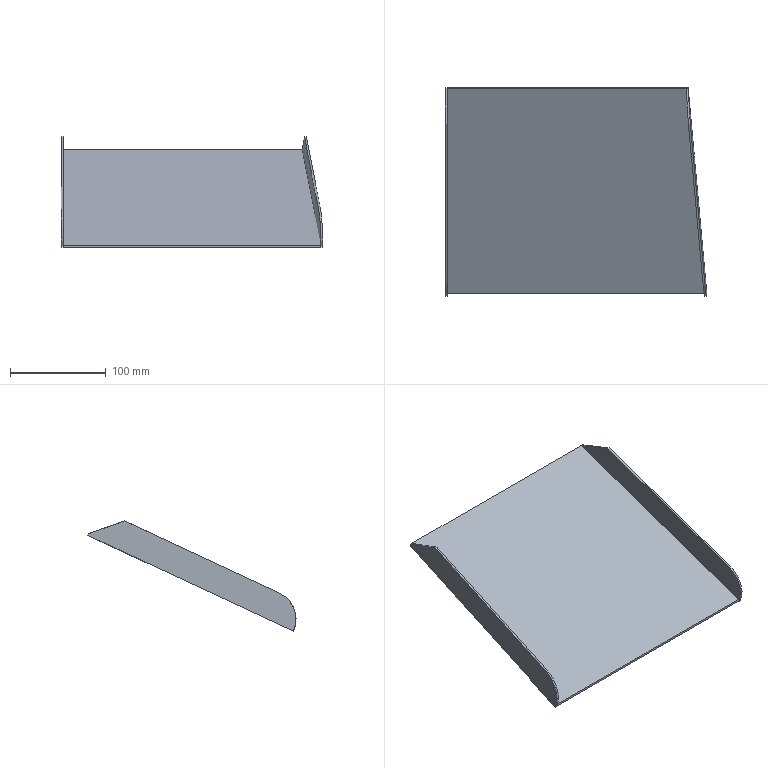Part | NX | features solid 2 | 1 solid | 15 faces | box 273.716 x 217.701 x 115.597 mm | volume 149004 mm3 | plane 12 | cylinder 2 | spline 1 | commonest cylinder face diameters 60 x2
STEP:
#1=CARTESIAN_POINT('',(382.,-625.361,-199.495));
#2=VERTEX_POINT('',#1);
#3=CARTESIAN_POINT('',(634.106,-625.268,-199.451));
#4=VERTEX_POINT('',#3);
#5=CARTESIAN_POINT('',(634.106,-625.268,-199.451));
#6=CARTESIAN_POINT('',(548.539,-625.34,-199.485));
#7=CARTESIAN_POINT('',(464.504,-625.371,-199.499));
#8=CARTESIAN_POINT('',(382.,-625.361,-199.495));
#9=B_SPLINE_CURVE_WITH_KNOTS('',3,(#5,#6,#7,#8),.UNSPECIFIED.,.F.,.F.,(4,4),(0.,0.992),.UNSPECIFIED.);
#10=EDGE_CURVE('',#2,#4,#9,.F.);
#11=ORIENTED_EDGE('',*,*,#10,.F.);
#12=CARTESIAN_POINT('',(382.,-626.207,-197.682));
#13=VERTEX_POINT('',#12);
#14=CARTESIAN_POINT('',(382.,-626.206,-197.682));
#15=CARTESIAN_POINT('',(382.,-625.925,-198.286));
#16=CARTESIAN_POINT('',(382.,-625.643,-198.89));
#17=CARTESIAN_POINT('',(382.,-625.361,-199.495));
#18=B_SPLINE_CURVE_WITH_KNOTS('',3,(#14,#15,#16,#17),.UNSPECIFIED.,.F.,.F.,(4,4),(0.,1.),.UNSPECIFIED.);
#19=EDGE_CURVE('',#2,#13,#18,.F.);
#20=ORIENTED_EDGE('',*,*,#19,.T.);
#21=CARTESIAN_POINT('',(634.106,-626.113,-197.638));
#22=VERTEX_POINT('',#21);
#23=CARTESIAN_POINT('',(634.106,-626.113,-197.638));
#24=CARTESIAN_POINT('',(548.539,-626.185,-197.672));
#25=CARTESIAN_POINT('',(464.504,-626.217,-197.687));
#26=CARTESIAN_POINT('',(382.,-626.207,-197.682));
#27=B_SPLINE_CURVE_WITH_KNOTS('',3,(#23,#24,#25,#26),.UNSPECIFIED.,.F.,.F.,(4,4),(0.,0.992),.UNSPECIFIED.);
#28=EDGE_CURVE('',#13,#22,#27,.F.);
#29=ORIENTED_EDGE('',*,*,#28,.T.);
#30=CARTESIAN_POINT('',(634.106,-625.268,-199.451));
#31=CARTESIAN_POINT('',(634.106,-625.55,-198.847));
#32=CARTESIAN_POINT('',(634.106,-625.831,-198.243));
#33=CARTESIAN_POINT('',(634.106,-626.113,-197.638));
#34=B_SPLINE_CURVE_WITH_KNOTS('',3,(#30,#31,#32,#33),.UNSPECIFIED.,.F.,.F.,(4,4),(0.,1.),.UNSPECIFIED.);
#35=EDGE_CURVE('',#22,#4,#34,.F.);
#36=ORIENTED_EDGE('',*,*,#35,.T.);
#37=EDGE_LOOP('',(#11,#20,#29,#36));
#38=FACE_BOUND('',#37,.T.);
#39=CARTESIAN_POINT('',(634.106,-626.113,-197.638));
#40=CARTESIAN_POINT('',(634.106,-625.268,-199.451));
#41=CARTESIAN_POINT('',(548.539,-626.185,-197.672));
#42=CARTESIAN_POINT('',(548.539,-625.34,-199.485));
#43=CARTESIAN_POINT('',(464.504,-626.217,-197.687));
#44=CARTESIAN_POINT('',(464.504,-625.371,-199.499));
#45=CARTESIAN_POINT('',(382.,-626.207,-197.682));
#46=CARTESIAN_POINT('',(382.,-625.361,-199.495));
#47=B_SPLINE_SURFACE_WITH_KNOTS('',3,1,((#39,#40),(#41,#42),(#43,#44),(#45,#46)),.SURF_OF_LINEAR_EXTRUSION.,.F.,.F.,.F.,(4,4),(2,2),(0.,0.992),(0.,1.),.PIECEWISE_BEZIER_KNOTS.);
#48=ADVANCED_FACE('',(#38),#47,.F.);
#49=CARTESIAN_POINT('',(382.,-840.,-299.582));
#50=VERTEX_POINT('',#49);
#51=CARTESIAN_POINT('',(382.,-840.,-297.376));
#52=VERTEX_POINT('',#51);
#53=CARTESIAN_POINT('',(382.,-840.,-720.));
#54=DIRECTION('',(0.,0.,1.));
#55=VECTOR('',#54,1000.);
#56=LINE('',#53,#55);
#57=EDGE_CURVE('',#50,#52,#56,.T.);
#58=ORIENTED_EDGE('',*,*,#57,.F.);
#59=CARTESIAN_POINT('',(651.709,-840.,-299.582));
#60=VERTEX_POINT('',#59);
#61=CARTESIAN_POINT('',(-476.248,-840.,-299.582));
#62=DIRECTION('',(1.,0.,0.));
#63=VECTOR('',#62,1000.);
#64=LINE('',#61,#63);
#65=EDGE_CURVE('',#50,#60,#64,.T.);
#66=ORIENTED_EDGE('',*,*,#65,.T.);
#67=CARTESIAN_POINT('',(651.632,-840.,-297.376));
#68=VERTEX_POINT('',#67);
#69=CARTESIAN_POINT('',(665.018,-840.,-680.08));
#70=DIRECTION('',(-0.03496,0.,0.9994));
#71=VECTOR('',#70,1000.);
#72=LINE('',#69,#71);
#73=EDGE_CURVE('',#60,#68,#72,.T.);
#74=ORIENTED_EDGE('',*,*,#73,.T.);
#75=CARTESIAN_POINT('',(-476.248,-840.,-297.376));
#76=DIRECTION('',(1.,0.,0.));
#77=VECTOR('',#76,1000.);
#78=LINE('',#75,#77);
#79=EDGE_CURVE('',#52,#68,#78,.T.);
#80=ORIENTED_EDGE('',*,*,#79,.F.);
#81=EDGE_LOOP('',(#58,#66,#74,#80));
#82=FACE_BOUND('',#81,.T.);
#83=CARTESIAN_POINT('',(-476.248,-840.,-720.));
#84=DIRECTION('',(0.,1.,0.));
#85=DIRECTION('',(-1.,0.,0.));
#86=AXIS2_PLACEMENT_3D('',#83,#84,#85);
#87=PLANE('',#86);
#88=ADVANCED_FACE('',(#82),#87,.F.);
#89=ORIENTED_EDGE('',*,*,#28,.F.);
#90=CARTESIAN_POINT('',(382.,-651.161,-209.318));
#91=DIRECTION('',(0.,-0.9063,-0.4226));
#92=VECTOR('',#91,1000.);
#93=LINE('',#90,#92);
#94=EDGE_CURVE('',#13,#52,#93,.T.);
#95=ORIENTED_EDGE('',*,*,#94,.T.);
#96=ORIENTED_EDGE('',*,*,#79,.T.);
#97=CARTESIAN_POINT('',(632.113,-626.263,-197.708));
#98=VERTEX_POINT('',#97);
#99=CARTESIAN_POINT('',(621.843,-513.811,-145.271));
#100=DIRECTION('',(0.08249,-0.9032,-0.4212));
#101=VECTOR('',#100,1000.);
#102=LINE('',#99,#101);
#103=EDGE_CURVE('',#98,#68,#102,.T.);
#104=ORIENTED_EDGE('',*,*,#103,.F.);
#105=CARTESIAN_POINT('',(634.106,-626.113,-197.638));
#106=DIRECTION('',(0.9966,0.07476,0.03486));
#107=VECTOR('',#106,1000.);
#108=LINE('',#105,#107);
#109=EDGE_CURVE('',#98,#22,#108,.T.);
#110=ORIENTED_EDGE('',*,*,#109,.T.);
#111=EDGE_LOOP('',(#89,#95,#96,#104,#110));
#112=FACE_BOUND('',#111,.T.);
#113=CARTESIAN_POINT('',(-1209.175,-651.161,-209.318));
#114=DIRECTION('',(0.,-0.4226,0.9063));
#115=DIRECTION('',(1.,0.,0.));
#116=AXIS2_PLACEMENT_3D('',#113,#114,#115);
#117=PLANE('',#116);
#118=ADVANCED_FACE('',(#112),#117,.T.);
#119=CARTESIAN_POINT('',(651.241,-825.582,-259.758));
#120=VERTEX_POINT('',#119);
#121=CARTESIAN_POINT('',(653.716,-840.,-299.582));
#122=VERTEX_POINT('',#121);
#123=CARTESIAN_POINT('',(651.241,-812.903,-286.947));
#124=DIRECTION('',(-0.9966,-0.07476,-0.03486));
#125=DIRECTION('',(0.0748,-0.9972,0.));
#126=AXIS2_PLACEMENT_3D('',#123,#124,#125);
#127=CIRCLE('',#126,30.);
#128=EDGE_CURVE('',#120,#122,#127,.F.);
#129=ORIENTED_EDGE('',*,*,#128,.T.);
#130=CARTESIAN_POINT('',(623.836,-512.816,-147.014));
#131=DIRECTION('',(0.08249,-0.9032,-0.4212));
#132=VECTOR('',#131,1000.);
#133=LINE('',#130,#132);
#134=EDGE_CURVE('',#4,#122,#133,.T.);
#135=ORIENTED_EDGE('',*,*,#134,.F.);
#136=ORIENTED_EDGE('',*,*,#35,.F.);
#137=CARTESIAN_POINT('',(636.415,-663.237,-184.055));
#138=VERTEX_POINT('',#137);
#139=CARTESIAN_POINT('',(636.415,-663.237,-184.055));
#140=DIRECTION('',(-0.05833,0.9375,-0.343));
#141=VECTOR('',#140,1000.);
#142=LINE('',#139,#141);
#143=EDGE_CURVE('',#22,#138,#142,.F.);
#144=ORIENTED_EDGE('',*,*,#143,.T.);
#145=CARTESIAN_POINT('',(634.106,-637.946,-172.262));
#146=DIRECTION('',(0.08249,-0.9032,-0.4212));
#147=VECTOR('',#146,1000.);
#148=LINE('',#145,#147);
#149=EDGE_CURVE('',#138,#120,#148,.T.);
#150=ORIENTED_EDGE('',*,*,#149,.T.);
#151=EDGE_LOOP('',(#129,#135,#136,#144,#150));
#152=FACE_BOUND('',#151,.T.);
#153=CARTESIAN_POINT('',(623.836,-513.661,-145.201));
#154=DIRECTION('',(0.9966,0.07476,0.03486));
#155=DIRECTION('',(-0.0748,0.9972,0.));
#156=AXIS2_PLACEMENT_3D('',#153,#154,#155);
#157=PLANE('',#156);
#158=ADVANCED_FACE('',(#152),#157,.T.);
#159=CARTESIAN_POINT('',(380.,-625.361,-199.495));
#160=VERTEX_POINT('',#159);
#161=CARTESIAN_POINT('',(380.,-840.,-299.582));
#162=VERTEX_POINT('',#161);
#163=CARTESIAN_POINT('',(380.,-650.315,-211.131));
#164=DIRECTION('',(0.,-0.9063,-0.4226));
#165=VECTOR('',#164,1000.);
#166=LINE('',#163,#165);
#167=EDGE_CURVE('',#160,#162,#166,.T.);
#168=ORIENTED_EDGE('',*,*,#167,.T.);
#169=CARTESIAN_POINT('',(380.,-825.489,-259.715));
#170=VERTEX_POINT('',#169);
#171=CARTESIAN_POINT('',(380.,-812.811,-286.904));
#172=DIRECTION('',(-1.,0.,0.));
#173=DIRECTION('',(0.,-1.,0.));
#174=AXIS2_PLACEMENT_3D('',#171,#172,#173);
#175=CIRCLE('',#174,30.);
#176=EDGE_CURVE('',#162,#170,#175,.T.);
#177=ORIENTED_EDGE('',*,*,#176,.T.);
#178=CARTESIAN_POINT('',(380.,-663.416,-184.139));
#179=VERTEX_POINT('',#178);
#180=CARTESIAN_POINT('',(380.,-638.04,-172.305));
#181=DIRECTION('',(0.,-0.9063,-0.4226));
#182=VECTOR('',#181,1000.);
#183=LINE('',#180,#182);
#184=EDGE_CURVE('',#179,#170,#183,.T.);
#185=ORIENTED_EDGE('',*,*,#184,.F.);
#186=CARTESIAN_POINT('',(380.,-626.206,-197.682));
#187=VERTEX_POINT('',#186);
#188=CARTESIAN_POINT('',(380.,-624.877,-198.166));
#189=DIRECTION('',(0.,-0.9397,0.342));
#190=VECTOR('',#189,1000.);
#191=LINE('',#188,#190);
#192=EDGE_CURVE('',#179,#187,#191,.F.);
#193=ORIENTED_EDGE('',*,*,#192,.T.);
#194=CARTESIAN_POINT('',(380.,-626.206,-197.682));
#195=CARTESIAN_POINT('',(380.,-625.925,-198.286));
#196=CARTESIAN_POINT('',(380.,-625.643,-198.89));
#197=CARTESIAN_POINT('',(380.,-625.361,-199.495));
#198=B_SPLINE_CURVE_WITH_KNOTS('',3,(#194,#195,#196,#197),.UNSPECIFIED.,.F.,.F.,(4,4),(0.,1.),.UNSPECIFIED.);
#199=EDGE_CURVE('',#160,#187,#198,.F.);
#200=ORIENTED_EDGE('',*,*,#199,.F.);
#201=EDGE_LOOP('',(#168,#177,#185,#193,#200));
#202=FACE_BOUND('',#201,.T.);
#203=CARTESIAN_POINT('',(380.,-651.161,-209.318));
#204=DIRECTION('',(1.,0.,0.));
#205=DIRECTION('',(0.,1.,0.));
#206=AXIS2_PLACEMENT_3D('',#203,#204,#205);
#207=PLANE('',#206);
#208=ADVANCED_FACE('',(#202),#207,.F.);
#209=CARTESIAN_POINT('',(382.,-625.361,-199.495));
#210=CARTESIAN_POINT('',(381.333,-625.361,-199.495));
#211=CARTESIAN_POINT('',(380.667,-625.361,-199.495));
#212=CARTESIAN_POINT('',(380.,-625.361,-199.495));
#213=B_SPLINE_CURVE_WITH_KNOTS('',3,(#209,#210,#211,#212),.UNSPECIFIED.,.F.,.F.,(4,4),(0.992,1.),.UNSPECIFIED.);
#214=EDGE_CURVE('',#160,#2,#213,.F.);
#215=ORIENTED_EDGE('',*,*,#214,.T.);
#216=ORIENTED_EDGE('',*,*,#10,.T.);
#217=ORIENTED_EDGE('',*,*,#134,.T.);
#218=CARTESIAN_POINT('',(651.723,-840.15,-299.652));
#219=VERTEX_POINT('',#218);
#220=CARTESIAN_POINT('',(653.716,-840.,-299.582));
#221=DIRECTION('',(0.9966,0.07476,0.03486));
#222=VECTOR('',#221,1000.);
#223=LINE('',#220,#222);
#224=EDGE_CURVE('',#122,#219,#223,.F.);
#225=ORIENTED_EDGE('',*,*,#224,.T.);
#226=CARTESIAN_POINT('',(632.113,-625.417,-199.521));
#227=DIRECTION('',(0.08249,-0.9032,-0.4212));
#228=VECTOR('',#227,1000.);
#229=LINE('',#226,#228);
#230=EDGE_CURVE('',#60,#219,#229,.T.);
#231=ORIENTED_EDGE('',*,*,#230,.F.);
#232=ORIENTED_EDGE('',*,*,#65,.F.);
#233=CARTESIAN_POINT('',(-476.248,-840.,-299.582));
#234=DIRECTION('',(1.,0.,0.));
#235=VECTOR('',#234,1000.);
#236=LINE('',#233,#235);
#237=EDGE_CURVE('',#162,#50,#236,.T.);
#238=ORIENTED_EDGE('',*,*,#237,.F.);
#239=ORIENTED_EDGE('',*,*,#167,.F.);
#240=EDGE_LOOP('',(#215,#216,#217,#225,#231,#232,#238,#239));
#241=FACE_BOUND('',#240,.T.);
#242=CARTESIAN_POINT('',(-1209.175,-650.315,-211.131));
#243=DIRECTION('',(0.,-0.4226,0.9063));
#244=DIRECTION('',(1.,0.,0.));
#245=AXIS2_PLACEMENT_3D('',#242,#243,#244);
#246=PLANE('',#245);
#247=ADVANCED_FACE('',(#241),#246,.F.);
#248=ORIENTED_EDGE('',*,*,#73,.F.);
#249=ORIENTED_EDGE('',*,*,#230,.T.);
#250=CARTESIAN_POINT('',(649.248,-825.731,-259.827));
#251=VERTEX_POINT('',#250);
#252=CARTESIAN_POINT('',(649.248,-813.053,-287.017));
#253=DIRECTION('',(-0.9966,-0.07476,-0.03486));
#254=DIRECTION('',(0.0748,-0.9972,0.));
#255=AXIS2_PLACEMENT_3D('',#252,#253,#254);
#256=CIRCLE('',#255,30.);
#257=EDGE_CURVE('',#219,#251,#256,.T.);
#258=ORIENTED_EDGE('',*,*,#257,.T.);
#259=CARTESIAN_POINT('',(634.422,-663.386,-184.125));
#260=VERTEX_POINT('',#259);
#261=CARTESIAN_POINT('',(632.113,-638.096,-172.332));
#262=DIRECTION('',(0.08249,-0.9032,-0.4212));
#263=VECTOR('',#262,1000.);
#264=LINE('',#261,#263);
#265=EDGE_CURVE('',#260,#251,#264,.T.);
#266=ORIENTED_EDGE('',*,*,#265,.F.);
#267=CARTESIAN_POINT('',(632.03,-624.937,-198.193));
#268=DIRECTION('',(0.05833,-0.9375,0.343));
#269=VECTOR('',#268,1000.);
#270=LINE('',#267,#269);
#271=EDGE_CURVE('',#260,#98,#270,.F.);
#272=ORIENTED_EDGE('',*,*,#271,.T.);
#273=ORIENTED_EDGE('',*,*,#103,.T.);
#274=EDGE_LOOP('',(#248,#249,#258,#266,#272,#273));
#275=FACE_BOUND('',#274,.T.);
#276=CARTESIAN_POINT('',(632.113,-625.417,-199.521));
#277=DIRECTION('',(-0.9966,-0.07476,-0.03486));
#278=DIRECTION('',(0.0748,-0.9972,0.));
#279=AXIS2_PLACEMENT_3D('',#276,#277,#278);
#280=PLANE('',#279);
#281=ADVANCED_FACE('',(#275),#280,.T.);
#282=ORIENTED_EDGE('',*,*,#265,.T.);
#283=CARTESIAN_POINT('',(651.241,-825.582,-259.758));
#284=DIRECTION('',(0.9966,0.07476,0.03486));
#285=VECTOR('',#284,1000.);
#286=LINE('',#283,#285);
#287=EDGE_CURVE('',#251,#120,#286,.T.);
#288=ORIENTED_EDGE('',*,*,#287,.T.);
#289=ORIENTED_EDGE('',*,*,#149,.F.);
#290=CARTESIAN_POINT('',(636.415,-663.237,-184.055));
#291=DIRECTION('',(-0.9966,-0.07476,-0.03486));
#292=VECTOR('',#291,1000.);
#293=LINE('',#290,#292);
#294=EDGE_CURVE('',#138,#260,#293,.T.);
#295=ORIENTED_EDGE('',*,*,#294,.T.);
#296=EDGE_LOOP('',(#282,#288,#289,#295));
#297=FACE_BOUND('',#296,.T.);
#298=CARTESIAN_POINT('',(634.106,-637.946,-172.262));
#299=DIRECTION('',(0.,0.4226,-0.9063));
#300=DIRECTION('',(0.08249,-0.9032,-0.4212));
#301=AXIS2_PLACEMENT_3D('',#298,#299,#300);
#302=PLANE('',#301);
#303=ADVANCED_FACE('',(#297),#302,.F.);
#304=ORIENTED_EDGE('',*,*,#143,.F.);
#305=ORIENTED_EDGE('',*,*,#109,.F.);
#306=ORIENTED_EDGE('',*,*,#271,.F.);
#307=ORIENTED_EDGE('',*,*,#294,.F.);
#308=EDGE_LOOP('',(#304,#305,#306,#307));
#309=FACE_BOUND('',#308,.T.);
#310=CARTESIAN_POINT('',(636.415,-663.237,-184.055));
#311=DIRECTION('',(0.05833,-0.3398,-0.9387));
#312=DIRECTION('',(0.,0.9403,-0.3404));
#313=AXIS2_PLACEMENT_3D('',#310,#311,#312);
#314=PLANE('',#313);
#315=ADVANCED_FACE('',(#309),#314,.F.);
#316=ORIENTED_EDGE('',*,*,#128,.F.);
#317=ORIENTED_EDGE('',*,*,#287,.F.);
#318=ORIENTED_EDGE('',*,*,#257,.F.);
#319=ORIENTED_EDGE('',*,*,#224,.F.);
#320=EDGE_LOOP('',(#316,#317,#318,#319));
#321=FACE_BOUND('',#320,.T.);
#322=CARTESIAN_POINT('',(651.241,-812.903,-286.947));
#323=DIRECTION('',(0.9966,0.07476,0.03486));
#324=DIRECTION('',(-0.0748,0.9972,0.));
#325=AXIS2_PLACEMENT_3D('',#322,#323,#324);
#326=CYLINDRICAL_SURFACE('',#325,30.);
#327=ADVANCED_FACE('',(#321),#326,.T.);
#328=CARTESIAN_POINT('',(382.,-825.489,-259.715));
#329=VERTEX_POINT('',#328);
#330=CARTESIAN_POINT('',(382.,-812.811,-286.904));
#331=DIRECTION('',(-1.,0.,0.));
#332=DIRECTION('',(0.,-1.,0.));
#333=AXIS2_PLACEMENT_3D('',#330,#331,#332);
#334=CIRCLE('',#333,30.);
#335=EDGE_CURVE('',#329,#50,#334,.F.);
#336=ORIENTED_EDGE('',*,*,#335,.T.);
#337=ORIENTED_EDGE('',*,*,#57,.T.);
#338=ORIENTED_EDGE('',*,*,#94,.F.);
#339=CARTESIAN_POINT('',(382.,-663.416,-184.139));
#340=VERTEX_POINT('',#339);
#341=CARTESIAN_POINT('',(382.,-626.206,-197.682));
#342=DIRECTION('',(0.,0.9397,-0.342));
#343=VECTOR('',#342,1000.);
#344=LINE('',#341,#343);
#345=EDGE_CURVE('',#13,#340,#344,.F.);
#346=ORIENTED_EDGE('',*,*,#345,.T.);
#347=CARTESIAN_POINT('',(382.,-638.04,-172.305));
#348=DIRECTION('',(0.,-0.9063,-0.4226));
#349=VECTOR('',#348,1000.);
#350=LINE('',#347,#349);
#351=EDGE_CURVE('',#340,#329,#350,.T.);
#352=ORIENTED_EDGE('',*,*,#351,.T.);
#353=EDGE_LOOP('',(#336,#337,#338,#346,#352));
#354=FACE_BOUND('',#353,.T.);
#355=CARTESIAN_POINT('',(382.,-625.361,-199.495));
#356=DIRECTION('',(-1.,0.,0.));
#357=DIRECTION('',(0.,-1.,0.));
#358=AXIS2_PLACEMENT_3D('',#355,#356,#357);
#359=PLANE('',#358);
#360=ADVANCED_FACE('',(#354),#359,.F.);
#361=ORIENTED_EDGE('',*,*,#199,.T.);
#362=CARTESIAN_POINT('',(380.,-626.206,-197.682));
#363=DIRECTION('',(-1.,0.,0.));
#364=VECTOR('',#363,1000.);
#365=LINE('',#362,#364);
#366=EDGE_CURVE('',#187,#13,#365,.F.);
#367=ORIENTED_EDGE('',*,*,#366,.T.);
#368=ORIENTED_EDGE('',*,*,#19,.F.);
#369=ORIENTED_EDGE('',*,*,#214,.F.);
#370=EDGE_LOOP('',(#361,#367,#368,#369));
#371=FACE_BOUND('',#370,.T.);
#372=CARTESIAN_POINT('',(380.,-625.361,-199.495));
#373=DIRECTION('',(0.,-0.9063,-0.4226));
#374=DIRECTION('',(0.,-0.4226,0.9063));
#375=AXIS2_PLACEMENT_3D('',#372,#373,#374);
#376=PLANE('',#375);
#377=ADVANCED_FACE('',(#371),#376,.F.);
#378=ORIENTED_EDGE('',*,*,#184,.T.);
#379=CARTESIAN_POINT('',(380.,-825.489,-259.715));
#380=DIRECTION('',(1.,0.,0.));
#381=VECTOR('',#380,1000.);
#382=LINE('',#379,#381);
#383=EDGE_CURVE('',#170,#329,#382,.T.);
#384=ORIENTED_EDGE('',*,*,#383,.T.);
#385=ORIENTED_EDGE('',*,*,#351,.F.);
#386=CARTESIAN_POINT('',(380.,-663.416,-184.139));
#387=DIRECTION('',(1.,0.,0.));
#388=VECTOR('',#387,1000.);
#389=LINE('',#386,#388);
#390=EDGE_CURVE('',#340,#179,#389,.F.);
#391=ORIENTED_EDGE('',*,*,#390,.T.);
#392=EDGE_LOOP('',(#378,#384,#385,#391));
#393=FACE_BOUND('',#392,.T.);
#394=CARTESIAN_POINT('',(380.,-638.04,-172.305));
#395=DIRECTION('',(0.,0.4226,-0.9063));
#396=DIRECTION('',(0.,-0.9063,-0.4226));
#397=AXIS2_PLACEMENT_3D('',#394,#395,#396);
#398=PLANE('',#397);
#399=ADVANCED_FACE('',(#393),#398,.F.);
#400=ORIENTED_EDGE('',*,*,#192,.F.);
#401=ORIENTED_EDGE('',*,*,#390,.F.);
#402=ORIENTED_EDGE('',*,*,#345,.F.);
#403=ORIENTED_EDGE('',*,*,#366,.F.);
#404=EDGE_LOOP('',(#400,#401,#402,#403));
#405=FACE_BOUND('',#404,.T.);
#406=CARTESIAN_POINT('',(380.,-626.206,-197.682));
#407=DIRECTION('',(0.,-0.342,-0.9397));
#408=DIRECTION('',(0.,0.9397,-0.342));
#409=AXIS2_PLACEMENT_3D('',#406,#407,#408);
#410=PLANE('',#409);
#411=ADVANCED_FACE('',(#405),#410,.F.);
#412=ORIENTED_EDGE('',*,*,#176,.F.);
#413=ORIENTED_EDGE('',*,*,#237,.T.);
#414=ORIENTED_EDGE('',*,*,#335,.F.);
#415=ORIENTED_EDGE('',*,*,#383,.F.);
#416=EDGE_LOOP('',(#412,#413,#414,#415));
#417=FACE_BOUND('',#416,.T.);
#418=CARTESIAN_POINT('',(380.,-812.811,-286.904));
#419=DIRECTION('',(-1.,0.,0.));
#420=DIRECTION('',(0.,-1.,0.));
#421=AXIS2_PLACEMENT_3D('',#418,#419,#420);
#422=CYLINDRICAL_SURFACE('',#421,30.);
#423=ADVANCED_FACE('',(#417),#422,.T.);
#424=CLOSED_SHELL('',(#48,#88,#118,#158,#208,#247,#281,#303,#315,#327,#360,#377,#399,#411,#423));
#425=MANIFOLD_SOLID_BREP('',#424);
#426=(LENGTH_UNIT()NAMED_UNIT(*)SI_UNIT(.MILLI.,.METRE.));
#427=UNCERTAINTY_MEASURE_WITH_UNIT(LENGTH_MEASURE(0.0508),#426,'','');
#428=(NAMED_UNIT(*)PLANE_ANGLE_UNIT()SI_UNIT($,.RADIAN.));
#429=(NAMED_UNIT(*)SI_UNIT($,.STERADIAN.)SOLID_ANGLE_UNIT());
#430=(GEOMETRIC_REPRESENTATION_CONTEXT(3)GLOBAL_UNCERTAINTY_ASSIGNED_CONTEXT((#427))GLOBAL_UNIT_ASSIGNED_CONTEXT((#426,#428,#429))REPRESENTATION_CONTEXT('',''));
#431=ADVANCED_BREP_SHAPE_REPRESENTATION('',(#425),#430);